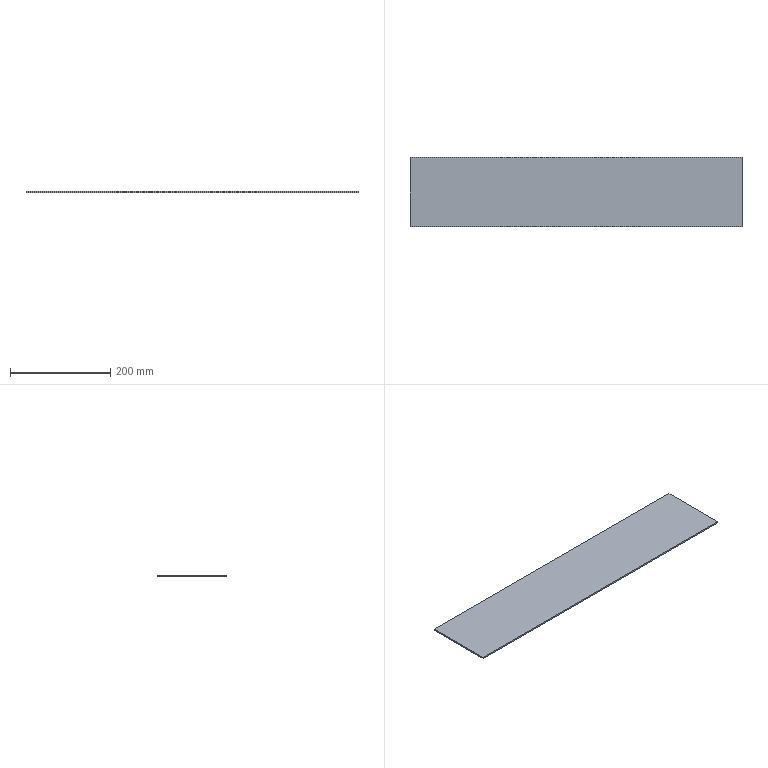Part | 1 solid | 6 faces | box 664 x 138 x 3 mm | volume 274896 mm3 | plane 6
STEP:
#1=CARTESIAN_POINT('',(332.,-69.,0.));
#2=VERTEX_POINT('',#1);
#3=CARTESIAN_POINT('',(332.,69.,0.));
#4=VERTEX_POINT('',#3);
#5=CARTESIAN_POINT('',(332.,69.,0.));
#6=DIRECTION('',(0.,1.,0.));
#7=VECTOR('',#6,1000.);
#8=LINE('',#5,#7);
#9=EDGE_CURVE('',#2,#4,#8,.T.);
#10=ORIENTED_EDGE('',*,*,#9,.T.);
#11=CARTESIAN_POINT('',(332.,69.,3.));
#12=VERTEX_POINT('',#11);
#13=CARTESIAN_POINT('',(332.,69.,3.));
#14=DIRECTION('',(0.,0.,-1.));
#15=VECTOR('',#14,1000.);
#16=LINE('',#13,#15);
#17=EDGE_CURVE('',#12,#4,#16,.T.);
#18=ORIENTED_EDGE('',*,*,#17,.F.);
#19=CARTESIAN_POINT('',(332.,-69.,3.));
#20=VERTEX_POINT('',#19);
#21=CARTESIAN_POINT('',(332.,69.,3.));
#22=DIRECTION('',(0.,1.,0.));
#23=VECTOR('',#22,1000.);
#24=LINE('',#21,#23);
#25=EDGE_CURVE('',#20,#12,#24,.T.);
#26=ORIENTED_EDGE('',*,*,#25,.F.);
#27=CARTESIAN_POINT('',(332.,-69.,3.));
#28=DIRECTION('',(0.,0.,-1.));
#29=VECTOR('',#28,1000.);
#30=LINE('',#27,#29);
#31=EDGE_CURVE('',#20,#2,#30,.T.);
#32=ORIENTED_EDGE('',*,*,#31,.T.);
#33=EDGE_LOOP('',(#10,#18,#26,#32));
#34=FACE_OUTER_BOUND('',#33,.T.);
#35=CARTESIAN_POINT('',(332.,69.,3.));
#36=DIRECTION('',(-1.,0.,0.));
#37=DIRECTION('',(0.,1.,0.));
#38=AXIS2_PLACEMENT_3D('',#35,#36,#37);
#39=PLANE('',#38);
#40=ADVANCED_FACE('',(#34),#39,.F.);
#41=CARTESIAN_POINT('',(-332.,69.,0.));
#42=VERTEX_POINT('',#41);
#43=CARTESIAN_POINT('',(-332.,69.,0.));
#44=DIRECTION('',(-1.,0.,0.));
#45=VECTOR('',#44,1000.);
#46=LINE('',#43,#45);
#47=EDGE_CURVE('',#4,#42,#46,.T.);
#48=ORIENTED_EDGE('',*,*,#47,.T.);
#49=CARTESIAN_POINT('',(-332.,69.,3.));
#50=VERTEX_POINT('',#49);
#51=CARTESIAN_POINT('',(-332.,69.,3.));
#52=DIRECTION('',(0.,0.,-1.));
#53=VECTOR('',#52,1000.);
#54=LINE('',#51,#53);
#55=EDGE_CURVE('',#50,#42,#54,.T.);
#56=ORIENTED_EDGE('',*,*,#55,.F.);
#57=CARTESIAN_POINT('',(-332.,69.,3.));
#58=DIRECTION('',(-1.,0.,0.));
#59=VECTOR('',#58,1000.);
#60=LINE('',#57,#59);
#61=EDGE_CURVE('',#12,#50,#60,.T.);
#62=ORIENTED_EDGE('',*,*,#61,.F.);
#63=ORIENTED_EDGE('',*,*,#17,.T.);
#64=EDGE_LOOP('',(#48,#56,#62,#63));
#65=FACE_OUTER_BOUND('',#64,.T.);
#66=CARTESIAN_POINT('',(-332.,69.,3.));
#67=DIRECTION('',(0.,-1.,0.));
#68=DIRECTION('',(0.,0.,-1.));
#69=AXIS2_PLACEMENT_3D('',#66,#67,#68);
#70=PLANE('',#69);
#71=ADVANCED_FACE('',(#65),#70,.F.);
#72=CARTESIAN_POINT('',(-332.,-69.,0.));
#73=VERTEX_POINT('',#72);
#74=CARTESIAN_POINT('',(-332.,69.,0.));
#75=DIRECTION('',(0.,-1.,0.));
#76=VECTOR('',#75,1000.);
#77=LINE('',#74,#76);
#78=EDGE_CURVE('',#42,#73,#77,.T.);
#79=ORIENTED_EDGE('',*,*,#78,.T.);
#80=CARTESIAN_POINT('',(-332.,-69.,3.));
#81=VERTEX_POINT('',#80);
#82=CARTESIAN_POINT('',(-332.,-69.,3.));
#83=DIRECTION('',(0.,0.,-1.));
#84=VECTOR('',#83,1000.);
#85=LINE('',#82,#84);
#86=EDGE_CURVE('',#81,#73,#85,.T.);
#87=ORIENTED_EDGE('',*,*,#86,.F.);
#88=CARTESIAN_POINT('',(-332.,69.,3.));
#89=DIRECTION('',(0.,-1.,0.));
#90=VECTOR('',#89,1000.);
#91=LINE('',#88,#90);
#92=EDGE_CURVE('',#50,#81,#91,.T.);
#93=ORIENTED_EDGE('',*,*,#92,.F.);
#94=ORIENTED_EDGE('',*,*,#55,.T.);
#95=EDGE_LOOP('',(#79,#87,#93,#94));
#96=FACE_OUTER_BOUND('',#95,.T.);
#97=CARTESIAN_POINT('',(-332.,69.,3.));
#98=DIRECTION('',(1.,0.,0.));
#99=DIRECTION('',(0.,1.,0.));
#100=AXIS2_PLACEMENT_3D('',#97,#98,#99);
#101=PLANE('',#100);
#102=ADVANCED_FACE('',(#96),#101,.F.);
#103=CARTESIAN_POINT('',(-332.,-69.,0.));
#104=DIRECTION('',(1.,0.,0.));
#105=VECTOR('',#104,1000.);
#106=LINE('',#103,#105);
#107=EDGE_CURVE('',#73,#2,#106,.T.);
#108=ORIENTED_EDGE('',*,*,#107,.T.);
#109=ORIENTED_EDGE('',*,*,#31,.F.);
#110=CARTESIAN_POINT('',(-332.,-69.,3.));
#111=DIRECTION('',(1.,0.,0.));
#112=VECTOR('',#111,1000.);
#113=LINE('',#110,#112);
#114=EDGE_CURVE('',#81,#20,#113,.T.);
#115=ORIENTED_EDGE('',*,*,#114,.F.);
#116=ORIENTED_EDGE('',*,*,#86,.T.);
#117=EDGE_LOOP('',(#108,#109,#115,#116));
#118=FACE_OUTER_BOUND('',#117,.T.);
#119=CARTESIAN_POINT('',(-332.,-69.,3.));
#120=DIRECTION('',(0.,1.,0.));
#121=DIRECTION('',(1.,0.,0.));
#122=AXIS2_PLACEMENT_3D('',#119,#120,#121);
#123=PLANE('',#122);
#124=ADVANCED_FACE('',(#118),#123,.F.);
#125=ORIENTED_EDGE('',*,*,#25,.T.);
#126=ORIENTED_EDGE('',*,*,#61,.T.);
#127=ORIENTED_EDGE('',*,*,#92,.T.);
#128=ORIENTED_EDGE('',*,*,#114,.T.);
#129=EDGE_LOOP('',(#125,#126,#127,#128));
#130=FACE_OUTER_BOUND('',#129,.T.);
#131=CARTESIAN_POINT('',(0.,0.,3.));
#132=DIRECTION('',(0.,0.,1.));
#133=DIRECTION('',(1.,0.,0.));
#134=AXIS2_PLACEMENT_3D('',#131,#132,#133);
#135=PLANE('',#134);
#136=ADVANCED_FACE('',(#130),#135,.T.);
#137=ORIENTED_EDGE('',*,*,#9,.F.);
#138=ORIENTED_EDGE('',*,*,#107,.F.);
#139=ORIENTED_EDGE('',*,*,#78,.F.);
#140=ORIENTED_EDGE('',*,*,#47,.F.);
#141=EDGE_LOOP('',(#137,#138,#139,#140));
#142=FACE_OUTER_BOUND('',#141,.T.);
#143=CARTESIAN_POINT('',(0.,0.,0.));
#144=DIRECTION('',(0.,0.,1.));
#145=DIRECTION('',(1.,0.,0.));
#146=AXIS2_PLACEMENT_3D('',#143,#144,#145);
#147=PLANE('',#146);
#148=ADVANCED_FACE('',(#142),#147,.F.);
#149=CLOSED_SHELL('',(#40,#71,#102,#124,#136,#148));
#150=MANIFOLD_SOLID_BREP('',#149);
#151=CARTESIAN_POINT('',(0.,0.,0.));
#152=DIRECTION('',(0.,0.,1.));
#153=DIRECTION('',(1.,0.,0.));
#154=AXIS2_PLACEMENT_3D('',#151,#152,#153);
#155=(LENGTH_UNIT()NAMED_UNIT(*)SI_UNIT(.MILLI.,.METRE.));
#156=UNCERTAINTY_MEASURE_WITH_UNIT(LENGTH_MEASURE(0.00001),#155,'','');
#157=(NAMED_UNIT(*)PLANE_ANGLE_UNIT()SI_UNIT($,.RADIAN.));
#158=(NAMED_UNIT(*)SI_UNIT($,.STERADIAN.)SOLID_ANGLE_UNIT());
#159=(GEOMETRIC_REPRESENTATION_CONTEXT(3)GLOBAL_UNCERTAINTY_ASSIGNED_CONTEXT((#156))GLOBAL_UNIT_ASSIGNED_CONTEXT((#155,#157,#158))REPRESENTATION_CONTEXT('',''));
#160=ADVANCED_BREP_SHAPE_REPRESENTATION('',(#150,#154),#159);